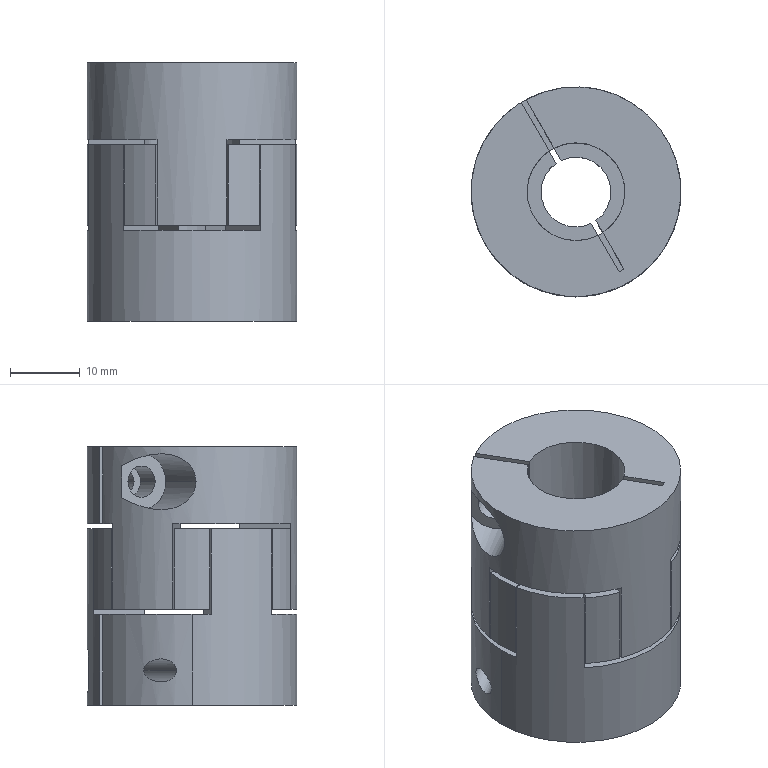Part | STEP file | coupling GHBG   LF-D-30-10-14 | 8 solids | 98 faces | box 30 x 30 x 37 mm | volume 19540 mm3 | plane 61 | cylinder 37 | commonest cylinder face diameters 14 x12 30 x11 3.3 x4 4.5 x4 8 x3 10 x3